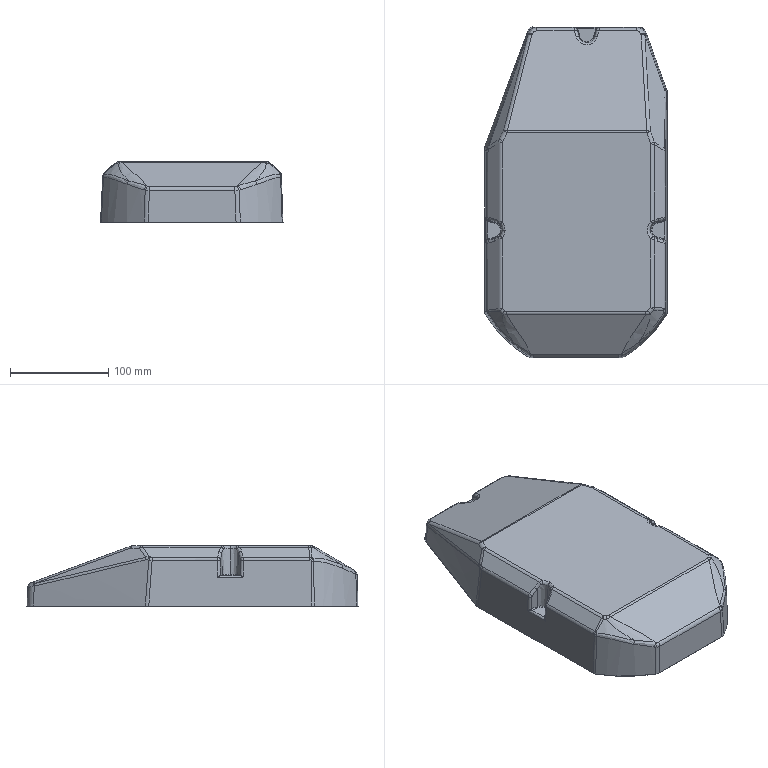Part | SolidWorks | features BaseBody 7, ICE 7 | 1 solid | 418 faces | box 186.614 x 338.671 x 61.577 mm | volume 394276 mm3 | spline 179 | cylinder 135 | plane 90 | cone 14 | commonest cylinder face diameters 10 x40 6 x28 16 x14 8 x9 2 x8 4 x6